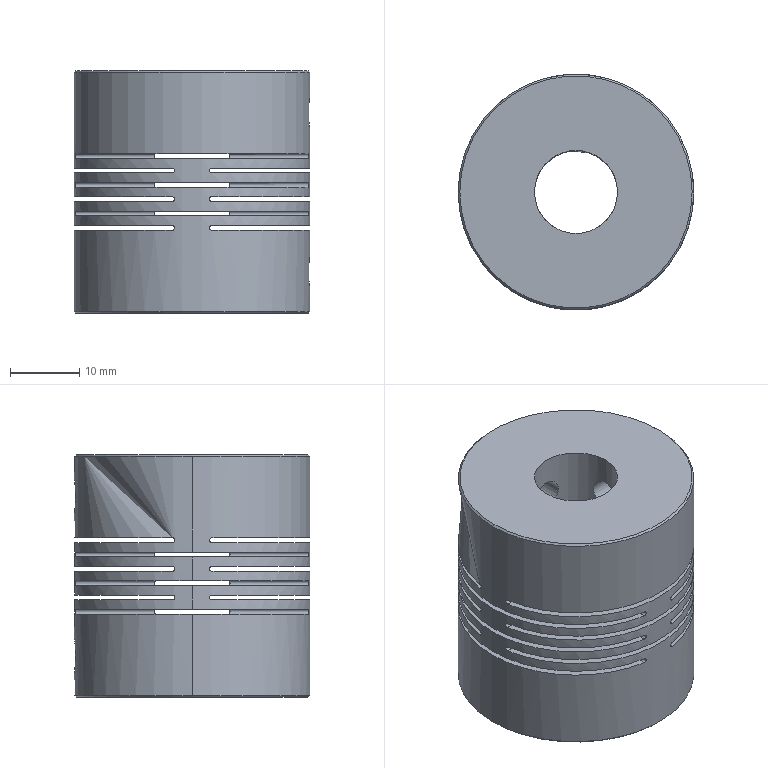Part | SolidWorks | features BaseBody 1 | 1 solid | 74 faces | box 34 x 34 x 35 mm | volume 24409 mm3 | cylinder 36 | plane 26 | cone 12 | commonest cylinder face diameters 0.688 x16 0.687 x8 4.134 x8 12 x2 34 x2